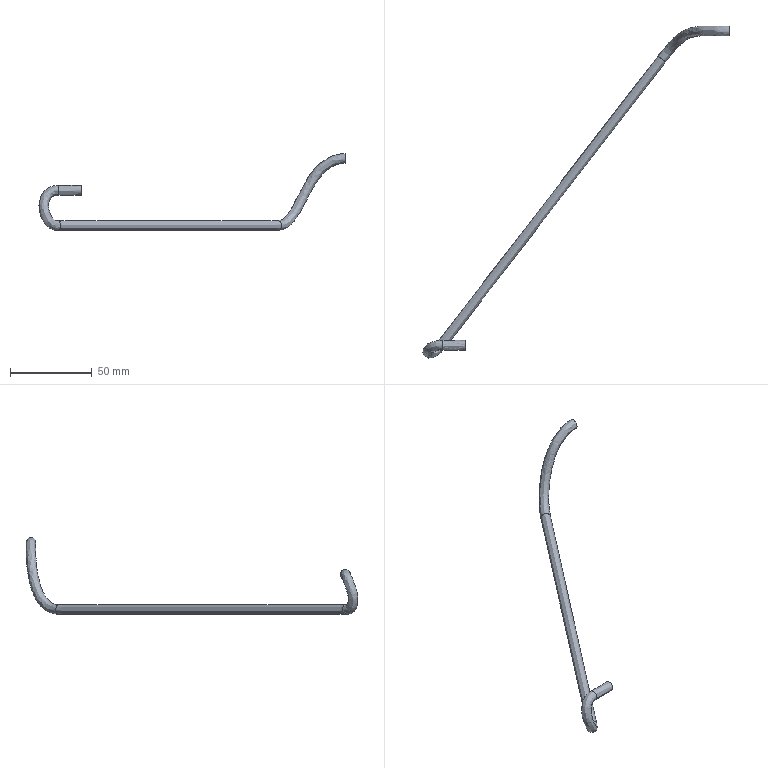Part | NX | features solid 2 | 1 solid | 10 faces | box 186.952 x 202.884 x 47.002 mm | volume 5271 mm3 | spline 8 | plane 2